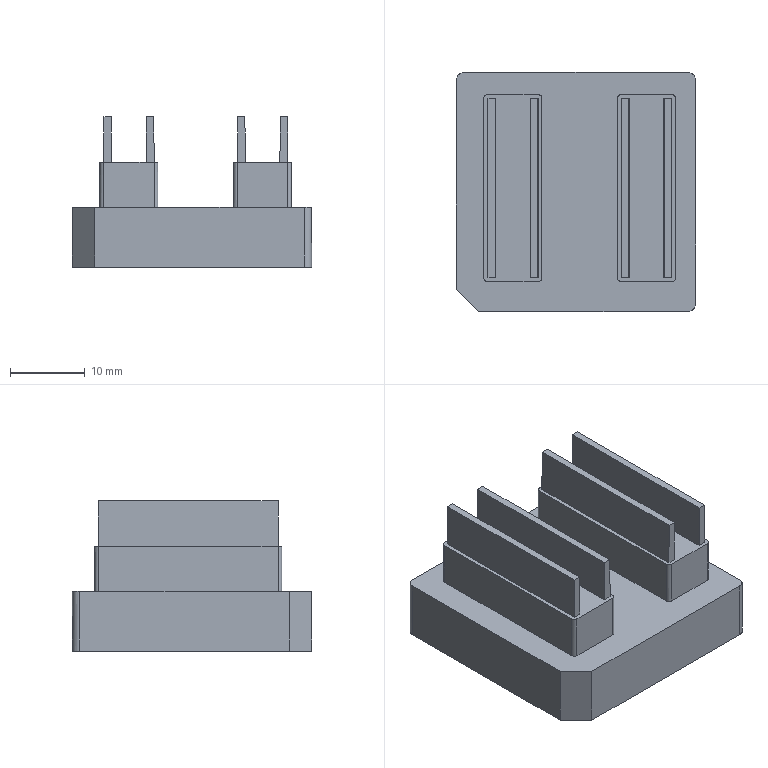CAM job | PowerMill | 3-axis milling, other | part box 32 x 32 x 20.109 mm
Tools:
number,name,type,diameter,tip_radius,length,cutting_length,overhang,flutes,holder,toolpaths_using
1,D10C,end_mill,10.0,0.0,60.0,,30.0,1,D42L35,1
1,D10C_1_1_1,end_mill,10.0,0.0,60.0,,20.56,1,D42L35,3
10,D3_1_1,end_mill,3.0,0.0,30.0,,12.28,1,D42L35,1
3,D10_1_1_1,end_mill,10.0,0.0,60.0,,20.28,1,D42L35,4
10,D3_2_1,end_mill,3.0,0.0,30.0,,6.32,1,D42L35,2
13,Text_D4_1_1,taper_spherical,4.0,0.3,60.0,,12.36,1,D42L35,1
Operations:
program,toolpath,strategy,tool,tool_number,tool_diameter,tip_radius,flutes,spindle_rpm,feed_cut,surface_speed_m_min_computed,feed_per_tooth_computed,tolerance,thickness,stepover,stepdown,cut_length,cut_time_min,total_time_min,workplane
11-C01-4-F,精公开粗01-扫面平行-D10C,raster_area_clear,D10C_1_1_1,1,10.0,0.0,1.0,8000.0,10000.0,251.33,1.25,0.03,0.28,6.0,1.0,338.04,0.034,0.04,
11-C01-4-F,精公开粗01-外形偏置-D10C,offset_area_clear,D10C_1_1_1,1,10.0,0.0,1.0,8000.0,10000.0,251.33,1.25,0.03,0.28,6.0,1.0,10328.196,1.033,1.111,
11-C01-4-F,精公开粗01-基准台等高-D10C,constantz,D10C_1_1_1,1,10.0,0.0,1.0,8000.0,10000.0,251.33,1.25,0.03,0.07,5.0,0.4,3449.049,0.345,0.3553,
11-C01-4-F,精公再粗02-外形偏置-D3,offset_area_clear,D3_1_1,10,3.0,0.0,1.0,18000.0,5000.0,169.65,0.2778,0.03,0.0,2.0,1.0,19719.592,3.944,4.578,
11-C01-4-F,精公基准台01-平坦面平行-D10,raster_area_clear,D10_1_1_1,3,10.0,0.0,1.0,8500.0,600.0,267.04,0.0706,0.005,0.38,5.0,1.0,224.962,0.375,0.409,
11-C01-4-F,精公基准台01-基准面偏置-D10,offset_area_clear,D10_1_1_1,3,10.0,0.0,1.0,8500.0,600.0,267.04,0.0706,0.005,0.38,5.0,1.0,144.172,0.24,0.2594,
11-C01-4-F,精公基准台01-外形侧光-D10,profile_area_clear,D10_1_1_1,3,10.0,0.0,1.0,8500.0,600.0,267.04,0.0706,0.005,-0.07,0.08,1.0,383.825,0.64,0.6802,
11-C01-4-F,精公基准台01-基准台侧光-D10,profile_area_clear,D10_1_1_1,3,10.0,0.0,1.0,8500.0,600.0,267.04,0.0706,0.005,0.0,0.08,1.0,313.234,0.522,0.5872,
11-C01-4-F,精公精光01-等高-D3,constantz,D3_2_1,10,3.0,0.0,1.0,18000.0,2000.0,169.65,0.1111,0.005,-0.075,5.0,0.02,35895.016,17.948,18.709,
11-C01-4-F,精公精光01-平坦面平行-D3,raster_area_clear,D3_2_1,10,3.0,0.0,1.0,18000.0,600.0,169.65,0.0333,0.005,0.375,1.5,1.0,672.339,1.12,1.272,
11-C01-4-F,精公刻字01-刻字-Text_D4,pattern,Text_D4_1_1,13,4.0,0.3,1.0,15000.0,1000.0,188.5,0.0667,0.005,0.0,5.0,1.0,46.32,0.046,0.0647,
,精公开粗01-外形偏置-D10C_Reference,offset_area_clear,D10C,1,10.0,0.0,1.0,8000.0,10000.0,251.33,1.25,0.03,0.28,6.0,1.0,26932.955,2.693,2.893,